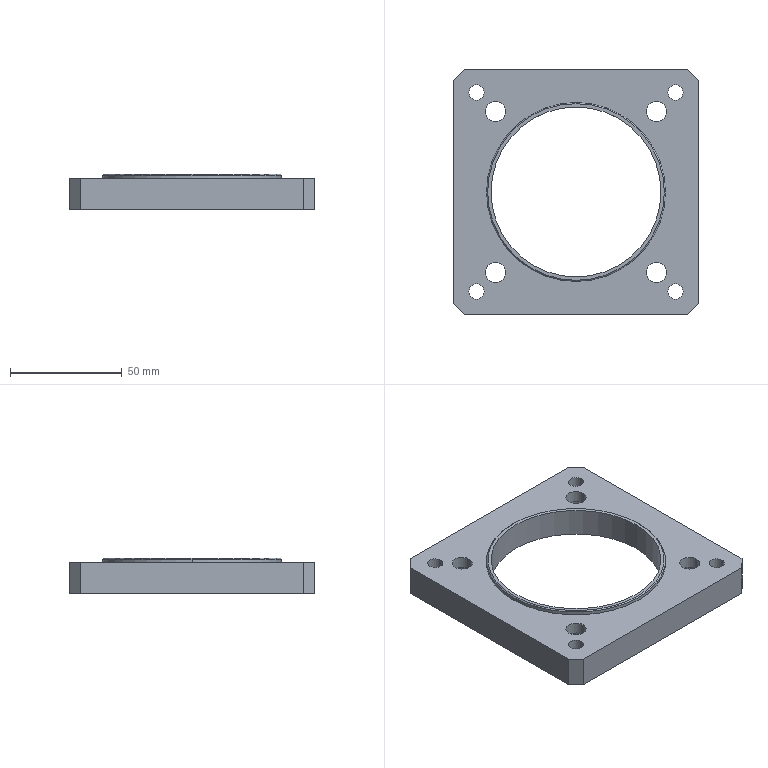Part | SolidWorks | features ICE 3, Chamfer 2, HoleWzd 2, Extrusion 1 | 1 solid | 50 faces | box 110 x 110 x 16 mm | volume 93090 mm3 | cylinder 30 | plane 16 | cone 4 | commonest cylinder face diameters 6.8 x8 9 x8 15 x8 76 x2 80 x2 85 x2
STEP:
#1=CARTESIAN_POINT('',(42.5,0.,0.5));
#2=VERTEX_POINT('',#1);
#3=CARTESIAN_POINT('',(-42.5,0.,0.5));
#4=VERTEX_POINT('',#3);
#5=CARTESIAN_POINT('',(0.,0.,0.5));
#6=DIRECTION('',(0.,0.,-1.));
#7=DIRECTION('',(-1.,0.,0.));
#8=AXIS2_PLACEMENT_3D('',#5,#6,#7);
#9=CIRCLE('',#8,42.5);
#10=EDGE_CURVE('',#2,#4,#9,.T.);
#11=ORIENTED_EDGE('',*,*,#10,.F.);
#12=CARTESIAN_POINT('',(43.,0.,0.));
#13=VERTEX_POINT('',#12);
#14=CARTESIAN_POINT('',(42.5,0.,0.5));
#15=DIRECTION('',(0.7071,0.,-0.7071));
#16=VECTOR('',#15,1000.);
#17=LINE('',#14,#16);
#18=EDGE_CURVE('',#2,#13,#17,.T.);
#19=ORIENTED_EDGE('',*,*,#18,.T.);
#20=CARTESIAN_POINT('',(-43.,0.,0.));
#21=VERTEX_POINT('',#20);
#22=CARTESIAN_POINT('',(0.,0.,0.));
#23=DIRECTION('',(0.,0.,1.));
#24=DIRECTION('',(-1.,0.,0.));
#25=AXIS2_PLACEMENT_3D('',#22,#23,#24);
#26=CIRCLE('',#25,43.);
#27=EDGE_CURVE('',#21,#13,#26,.T.);
#28=ORIENTED_EDGE('',*,*,#27,.F.);
#29=CARTESIAN_POINT('',(-42.5,0.,0.5));
#30=DIRECTION('',(-0.7071,0.,-0.7071));
#31=VECTOR('',#30,1000.);
#32=LINE('',#29,#31);
#33=EDGE_CURVE('',#4,#21,#32,.T.);
#34=ORIENTED_EDGE('',*,*,#33,.F.);
#35=EDGE_LOOP('',(#11,#19,#28,#34));
#36=FACE_OUTER_BOUND('',#35,.T.);
#37=CARTESIAN_POINT('',(0.,0.,0.5));
#38=DIRECTION('',(0.,0.,-1.));
#39=DIRECTION('',(-1.,0.,0.));
#40=AXIS2_PLACEMENT_3D('',#37,#38,#39);
#41=CONICAL_SURFACE('',#40,42.5,0.7854);
#42=ADVANCED_FACE('',(#36),#41,.F.);
#43=CARTESIAN_POINT('',(39.5,0.,16.));
#44=VERTEX_POINT('',#43);
#45=CARTESIAN_POINT('',(-39.5,0.,16.));
#46=VERTEX_POINT('',#45);
#47=CARTESIAN_POINT('',(0.,0.,16.));
#48=DIRECTION('',(0.,0.,1.));
#49=DIRECTION('',(1.,0.,0.));
#50=AXIS2_PLACEMENT_3D('',#47,#48,#49);
#51=CIRCLE('',#50,39.5);
#52=EDGE_CURVE('',#44,#46,#51,.T.);
#53=ORIENTED_EDGE('',*,*,#52,.F.);
#54=CARTESIAN_POINT('',(40.,0.,15.5));
#55=VERTEX_POINT('',#54);
#56=CARTESIAN_POINT('',(39.5,0.,16.));
#57=DIRECTION('',(0.7071,0.,-0.7071));
#58=VECTOR('',#57,1000.);
#59=LINE('',#56,#58);
#60=EDGE_CURVE('',#44,#55,#59,.T.);
#61=ORIENTED_EDGE('',*,*,#60,.T.);
#62=CARTESIAN_POINT('',(-40.,0.,15.5));
#63=VERTEX_POINT('',#62);
#64=CARTESIAN_POINT('',(0.,0.,15.5));
#65=DIRECTION('',(0.,0.,-1.));
#66=DIRECTION('',(1.,0.,0.));
#67=AXIS2_PLACEMENT_3D('',#64,#65,#66);
#68=CIRCLE('',#67,40.);
#69=EDGE_CURVE('',#63,#55,#68,.T.);
#70=ORIENTED_EDGE('',*,*,#69,.F.);
#71=CARTESIAN_POINT('',(-39.5,0.,16.));
#72=DIRECTION('',(-0.7071,0.,-0.7071));
#73=VECTOR('',#72,1000.);
#74=LINE('',#71,#73);
#75=EDGE_CURVE('',#46,#63,#74,.T.);
#76=ORIENTED_EDGE('',*,*,#75,.F.);
#77=EDGE_LOOP('',(#53,#61,#70,#76));
#78=FACE_OUTER_BOUND('',#77,.T.);
#79=CARTESIAN_POINT('',(0.,0.,16.));
#80=DIRECTION('',(0.,0.,-1.));
#81=DIRECTION('',(-1.,0.,0.));
#82=AXIS2_PLACEMENT_3D('',#79,#80,#81);
#83=CONICAL_SURFACE('',#82,39.5,0.7854);
#84=ADVANCED_FACE('',(#78),#83,.T.);
#85=CARTESIAN_POINT('',(-28.5,36.,8.6));
#86=VERTEX_POINT('',#85);
#87=CARTESIAN_POINT('',(-43.5,36.,8.6));
#88=VERTEX_POINT('',#87);
#89=CARTESIAN_POINT('',(-36.,36.,8.6));
#90=DIRECTION('',(0.,0.,-1.));
#91=DIRECTION('',(-1.,0.,0.));
#92=AXIS2_PLACEMENT_3D('',#89,#90,#91);
#93=CIRCLE('',#92,7.5);
#94=EDGE_CURVE('',#86,#88,#93,.T.);
#95=ORIENTED_EDGE('',*,*,#94,.F.);
#96=CARTESIAN_POINT('',(-28.5,36.,0.));
#97=VERTEX_POINT('',#96);
#98=CARTESIAN_POINT('',(-28.5,36.,0.));
#99=DIRECTION('',(0.,0.,-1.));
#100=VECTOR('',#99,1000.);
#101=LINE('',#98,#100);
#102=EDGE_CURVE('',#86,#97,#101,.T.);
#103=ORIENTED_EDGE('',*,*,#102,.T.);
#104=CARTESIAN_POINT('',(-43.5,36.,0.));
#105=VERTEX_POINT('',#104);
#106=CARTESIAN_POINT('',(-36.,36.,0.));
#107=DIRECTION('',(0.,0.,-1.));
#108=DIRECTION('',(-1.,0.,0.));
#109=AXIS2_PLACEMENT_3D('',#106,#107,#108);
#110=CIRCLE('',#109,7.5);
#111=EDGE_CURVE('',#97,#105,#110,.T.);
#112=ORIENTED_EDGE('',*,*,#111,.T.);
#113=CARTESIAN_POINT('',(-43.5,36.,0.));
#114=DIRECTION('',(0.,0.,-1.));
#115=VECTOR('',#114,1000.);
#116=LINE('',#113,#115);
#117=EDGE_CURVE('',#88,#105,#116,.T.);
#118=ORIENTED_EDGE('',*,*,#117,.F.);
#119=EDGE_LOOP('',(#95,#103,#112,#118));
#120=FACE_OUTER_BOUND('',#119,.T.);
#121=CARTESIAN_POINT('',(-36.,36.,0.));
#122=DIRECTION('',(0.,0.,-1.));
#123=DIRECTION('',(-1.,0.,0.));
#124=AXIS2_PLACEMENT_3D('',#121,#122,#123);
#125=CYLINDRICAL_SURFACE('',#124,7.5);
#126=ADVANCED_FACE('',(#120),#125,.F.);
#127=CARTESIAN_POINT('',(-31.5,36.,14.));
#128=VERTEX_POINT('',#127);
#129=CARTESIAN_POINT('',(-40.5,36.,14.));
#130=VERTEX_POINT('',#129);
#131=CARTESIAN_POINT('',(-36.,36.,14.));
#132=DIRECTION('',(0.,0.,-1.));
#133=DIRECTION('',(-1.,0.,0.));
#134=AXIS2_PLACEMENT_3D('',#131,#132,#133);
#135=CIRCLE('',#134,4.5);
#136=EDGE_CURVE('',#128,#130,#135,.T.);
#137=ORIENTED_EDGE('',*,*,#136,.F.);
#138=CARTESIAN_POINT('',(-31.5,36.,8.6));
#139=VERTEX_POINT('',#138);
#140=CARTESIAN_POINT('',(-31.5,36.,0.));
#141=DIRECTION('',(0.,0.,-1.));
#142=VECTOR('',#141,1000.);
#143=LINE('',#140,#142);
#144=EDGE_CURVE('',#128,#139,#143,.T.);
#145=ORIENTED_EDGE('',*,*,#144,.T.);
#146=CARTESIAN_POINT('',(-40.5,36.,8.6));
#147=VERTEX_POINT('',#146);
#148=CARTESIAN_POINT('',(-36.,36.,8.6));
#149=DIRECTION('',(0.,0.,-1.));
#150=DIRECTION('',(-1.,0.,0.));
#151=AXIS2_PLACEMENT_3D('',#148,#149,#150);
#152=CIRCLE('',#151,4.5);
#153=EDGE_CURVE('',#139,#147,#152,.T.);
#154=ORIENTED_EDGE('',*,*,#153,.T.);
#155=CARTESIAN_POINT('',(-40.5,36.,0.));
#156=DIRECTION('',(0.,0.,-1.));
#157=VECTOR('',#156,1000.);
#158=LINE('',#155,#157);
#159=EDGE_CURVE('',#130,#147,#158,.T.);
#160=ORIENTED_EDGE('',*,*,#159,.F.);
#161=EDGE_LOOP('',(#137,#145,#154,#160));
#162=FACE_OUTER_BOUND('',#161,.T.);
#163=CARTESIAN_POINT('',(-36.,36.,0.));
#164=DIRECTION('',(0.,0.,-1.));
#165=DIRECTION('',(-1.,0.,0.));
#166=AXIS2_PLACEMENT_3D('',#163,#164,#165);
#167=CYLINDRICAL_SURFACE('',#166,4.5);
#168=ADVANCED_FACE('',(#162),#167,.F.);
#169=CARTESIAN_POINT('',(43.5,-36.,8.6));
#170=VERTEX_POINT('',#169);
#171=CARTESIAN_POINT('',(28.5,-36.,8.6));
#172=VERTEX_POINT('',#171);
#173=CARTESIAN_POINT('',(36.,-36.,8.6));
#174=DIRECTION('',(0.,0.,-1.));
#175=DIRECTION('',(-1.,0.,0.));
#176=AXIS2_PLACEMENT_3D('',#173,#174,#175);
#177=CIRCLE('',#176,7.5);
#178=EDGE_CURVE('',#170,#172,#177,.T.);
#179=ORIENTED_EDGE('',*,*,#178,.F.);
#180=CARTESIAN_POINT('',(43.5,-36.,0.));
#181=VERTEX_POINT('',#180);
#182=CARTESIAN_POINT('',(43.5,-36.,0.));
#183=DIRECTION('',(0.,0.,-1.));
#184=VECTOR('',#183,1000.);
#185=LINE('',#182,#184);
#186=EDGE_CURVE('',#170,#181,#185,.T.);
#187=ORIENTED_EDGE('',*,*,#186,.T.);
#188=CARTESIAN_POINT('',(28.5,-36.,0.));
#189=VERTEX_POINT('',#188);
#190=CARTESIAN_POINT('',(36.,-36.,0.));
#191=DIRECTION('',(0.,0.,-1.));
#192=DIRECTION('',(-1.,0.,0.));
#193=AXIS2_PLACEMENT_3D('',#190,#191,#192);
#194=CIRCLE('',#193,7.5);
#195=EDGE_CURVE('',#181,#189,#194,.T.);
#196=ORIENTED_EDGE('',*,*,#195,.T.);
#197=CARTESIAN_POINT('',(28.5,-36.,0.));
#198=DIRECTION('',(0.,0.,-1.));
#199=VECTOR('',#198,1000.);
#200=LINE('',#197,#199);
#201=EDGE_CURVE('',#172,#189,#200,.T.);
#202=ORIENTED_EDGE('',*,*,#201,.F.);
#203=EDGE_LOOP('',(#179,#187,#196,#202));
#204=FACE_OUTER_BOUND('',#203,.T.);
#205=CARTESIAN_POINT('',(36.,-36.,0.));
#206=DIRECTION('',(0.,0.,-1.));
#207=DIRECTION('',(-1.,0.,0.));
#208=AXIS2_PLACEMENT_3D('',#205,#206,#207);
#209=CYLINDRICAL_SURFACE('',#208,7.5);
#210=ADVANCED_FACE('',(#204),#209,.F.);
#211=CARTESIAN_POINT('',(40.5,-36.,14.));
#212=VERTEX_POINT('',#211);
#213=CARTESIAN_POINT('',(31.5,-36.,14.));
#214=VERTEX_POINT('',#213);
#215=CARTESIAN_POINT('',(36.,-36.,14.));
#216=DIRECTION('',(0.,0.,-1.));
#217=DIRECTION('',(-1.,0.,0.));
#218=AXIS2_PLACEMENT_3D('',#215,#216,#217);
#219=CIRCLE('',#218,4.5);
#220=EDGE_CURVE('',#212,#214,#219,.T.);
#221=ORIENTED_EDGE('',*,*,#220,.F.);
#222=CARTESIAN_POINT('',(40.5,-36.,8.6));
#223=VERTEX_POINT('',#222);
#224=CARTESIAN_POINT('',(40.5,-36.,0.));
#225=DIRECTION('',(0.,0.,-1.));
#226=VECTOR('',#225,1000.);
#227=LINE('',#224,#226);
#228=EDGE_CURVE('',#212,#223,#227,.T.);
#229=ORIENTED_EDGE('',*,*,#228,.T.);
#230=CARTESIAN_POINT('',(31.5,-36.,8.6));
#231=VERTEX_POINT('',#230);
#232=CARTESIAN_POINT('',(36.,-36.,8.6));
#233=DIRECTION('',(0.,0.,-1.));
#234=DIRECTION('',(-1.,0.,0.));
#235=AXIS2_PLACEMENT_3D('',#232,#233,#234);
#236=CIRCLE('',#235,4.5);
#237=EDGE_CURVE('',#223,#231,#236,.T.);
#238=ORIENTED_EDGE('',*,*,#237,.T.);
#239=CARTESIAN_POINT('',(31.5,-36.,0.));
#240=DIRECTION('',(0.,0.,-1.));
#241=VECTOR('',#240,1000.);
#242=LINE('',#239,#241);
#243=EDGE_CURVE('',#214,#231,#242,.T.);
#244=ORIENTED_EDGE('',*,*,#243,.F.);
#245=EDGE_LOOP('',(#221,#229,#238,#244));
#246=FACE_OUTER_BOUND('',#245,.T.);
#247=CARTESIAN_POINT('',(36.,-36.,0.));
#248=DIRECTION('',(0.,0.,-1.));
#249=DIRECTION('',(-1.,0.,0.));
#250=AXIS2_PLACEMENT_3D('',#247,#248,#249);
#251=CYLINDRICAL_SURFACE('',#250,4.5);
#252=ADVANCED_FACE('',(#246),#251,.F.);
#253=CARTESIAN_POINT('',(43.5,36.,8.6));
#254=VERTEX_POINT('',#253);
#255=CARTESIAN_POINT('',(28.5,36.,8.6));
#256=VERTEX_POINT('',#255);
#257=CARTESIAN_POINT('',(36.,36.,8.6));
#258=DIRECTION('',(0.,0.,-1.));
#259=DIRECTION('',(-1.,0.,0.));
#260=AXIS2_PLACEMENT_3D('',#257,#258,#259);
#261=CIRCLE('',#260,7.5);
#262=EDGE_CURVE('',#254,#256,#261,.T.);
#263=ORIENTED_EDGE('',*,*,#262,.F.);
#264=CARTESIAN_POINT('',(43.5,36.,0.));
#265=VERTEX_POINT('',#264);
#266=CARTESIAN_POINT('',(43.5,36.,0.));
#267=DIRECTION('',(0.,0.,-1.));
#268=VECTOR('',#267,1000.);
#269=LINE('',#266,#268);
#270=EDGE_CURVE('',#254,#265,#269,.T.);
#271=ORIENTED_EDGE('',*,*,#270,.T.);
#272=CARTESIAN_POINT('',(28.5,36.,0.));
#273=VERTEX_POINT('',#272);
#274=CARTESIAN_POINT('',(36.,36.,0.));
#275=DIRECTION('',(0.,0.,-1.));
#276=DIRECTION('',(-1.,0.,0.));
#277=AXIS2_PLACEMENT_3D('',#274,#275,#276);
#278=CIRCLE('',#277,7.5);
#279=EDGE_CURVE('',#265,#273,#278,.T.);
#280=ORIENTED_EDGE('',*,*,#279,.T.);
#281=CARTESIAN_POINT('',(28.5,36.,0.));
#282=DIRECTION('',(0.,0.,-1.));
#283=VECTOR('',#282,1000.);
#284=LINE('',#281,#283);
#285=EDGE_CURVE('',#256,#273,#284,.T.);
#286=ORIENTED_EDGE('',*,*,#285,.F.);
#287=EDGE_LOOP('',(#263,#271,#280,#286));
#288=FACE_OUTER_BOUND('',#287,.T.);
#289=CARTESIAN_POINT('',(36.,36.,0.));
#290=DIRECTION('',(0.,0.,-1.));
#291=DIRECTION('',(-1.,0.,0.));
#292=AXIS2_PLACEMENT_3D('',#289,#290,#291);
#293=CYLINDRICAL_SURFACE('',#292,7.5);
#294=ADVANCED_FACE('',(#288),#293,.F.);
#295=CARTESIAN_POINT('',(40.5,36.,14.));
#296=VERTEX_POINT('',#295);
#297=CARTESIAN_POINT('',(31.5,36.,14.));
#298=VERTEX_POINT('',#297);
#299=CARTESIAN_POINT('',(36.,36.,14.));
#300=DIRECTION('',(0.,0.,-1.));
#301=DIRECTION('',(-1.,0.,0.));
#302=AXIS2_PLACEMENT_3D('',#299,#300,#301);
#303=CIRCLE('',#302,4.5);
#304=EDGE_CURVE('',#296,#298,#303,.T.);
#305=ORIENTED_EDGE('',*,*,#304,.F.);
#306=CARTESIAN_POINT('',(40.5,36.,8.6));
#307=VERTEX_POINT('',#306);
#308=CARTESIAN_POINT('',(40.5,36.,0.));
#309=DIRECTION('',(0.,0.,-1.));
#310=VECTOR('',#309,1000.);
#311=LINE('',#308,#310);
#312=EDGE_CURVE('',#296,#307,#311,.T.);
#313=ORIENTED_EDGE('',*,*,#312,.T.);
#314=CARTESIAN_POINT('',(31.5,36.,8.6));
#315=VERTEX_POINT('',#314);
#316=CARTESIAN_POINT('',(36.,36.,8.6));
#317=DIRECTION('',(0.,0.,-1.));
#318=DIRECTION('',(-1.,0.,0.));
#319=AXIS2_PLACEMENT_3D('',#316,#317,#318);
#320=CIRCLE('',#319,4.5);
#321=EDGE_CURVE('',#307,#315,#320,.T.);
#322=ORIENTED_EDGE('',*,*,#321,.T.);
#323=CARTESIAN_POINT('',(31.5,36.,0.));
#324=DIRECTION('',(0.,0.,-1.));
#325=VECTOR('',#324,1000.);
#326=LINE('',#323,#325);
#327=EDGE_CURVE('',#298,#315,#326,.T.);
#328=ORIENTED_EDGE('',*,*,#327,.F.);
#329=EDGE_LOOP('',(#305,#313,#322,#328));
#330=FACE_OUTER_BOUND('',#329,.T.);
#331=CARTESIAN_POINT('',(36.,36.,0.));
#332=DIRECTION('',(0.,0.,-1.));
#333=DIRECTION('',(-1.,0.,0.));
#334=AXIS2_PLACEMENT_3D('',#331,#332,#333);
#335=CYLINDRICAL_SURFACE('',#334,4.5);
#336=ADVANCED_FACE('',(#330),#335,.F.);
#337=CARTESIAN_POINT('',(-28.5,-36.,8.6));
#338=VERTEX_POINT('',#337);
#339=CARTESIAN_POINT('',(-43.5,-36.,8.6));
#340=VERTEX_POINT('',#339);
#341=CARTESIAN_POINT('',(-36.,-36.,8.6));
#342=DIRECTION('',(0.,0.,-1.));
#343=DIRECTION('',(-1.,0.,0.));
#344=AXIS2_PLACEMENT_3D('',#341,#342,#343);
#345=CIRCLE('',#344,7.5);
#346=EDGE_CURVE('',#338,#340,#345,.T.);
#347=ORIENTED_EDGE('',*,*,#346,.F.);
#348=CARTESIAN_POINT('',(-28.5,-36.,0.));
#349=VERTEX_POINT('',#348);
#350=CARTESIAN_POINT('',(-28.5,-36.,0.));
#351=DIRECTION('',(0.,0.,-1.));
#352=VECTOR('',#351,1000.);
#353=LINE('',#350,#352);
#354=EDGE_CURVE('',#338,#349,#353,.T.);
#355=ORIENTED_EDGE('',*,*,#354,.T.);
#356=CARTESIAN_POINT('',(-43.5,-36.,0.));
#357=VERTEX_POINT('',#356);
#358=CARTESIAN_POINT('',(-36.,-36.,0.));
#359=DIRECTION('',(0.,0.,-1.));
#360=DIRECTION('',(-1.,0.,0.));
#361=AXIS2_PLACEMENT_3D('',#358,#359,#360);
#362=CIRCLE('',#361,7.5);
#363=EDGE_CURVE('',#349,#357,#362,.T.);
#364=ORIENTED_EDGE('',*,*,#363,.T.);
#365=CARTESIAN_POINT('',(-43.5,-36.,0.));
#366=DIRECTION('',(0.,0.,-1.));
#367=VECTOR('',#366,1000.);
#368=LINE('',#365,#367);
#369=EDGE_CURVE('',#340,#357,#368,.T.);
#370=ORIENTED_EDGE('',*,*,#369,.F.);
#371=EDGE_LOOP('',(#347,#355,#364,#370));
#372=FACE_OUTER_BOUND('',#371,.T.);
#373=CARTESIAN_POINT('',(-36.,-36.,0.));
#374=DIRECTION('',(0.,0.,-1.));
#375=DIRECTION('',(-1.,0.,0.));
#376=AXIS2_PLACEMENT_3D('',#373,#374,#375);
#377=CYLINDRICAL_SURFACE('',#376,7.5);
#378=ADVANCED_FACE('',(#372),#377,.F.);
#379=CARTESIAN_POINT('',(-31.5,-36.,14.));
#380=VERTEX_POINT('',#379);
#381=CARTESIAN_POINT('',(-40.5,-36.,14.));
#382=VERTEX_POINT('',#381);
#383=CARTESIAN_POINT('',(-36.,-36.,14.));
#384=DIRECTION('',(0.,0.,-1.));
#385=DIRECTION('',(-1.,0.,0.));
#386=AXIS2_PLACEMENT_3D('',#383,#384,#385);
#387=CIRCLE('',#386,4.5);
#388=EDGE_CURVE('',#380,#382,#387,.T.);
#389=ORIENTED_EDGE('',*,*,#388,.F.);
#390=CARTESIAN_POINT('',(-31.5,-36.,8.6));
#391=VERTEX_POINT('',#390);
#392=CARTESIAN_POINT('',(-31.5,-36.,0.));
#393=DIRECTION('',(0.,0.,-1.));
#394=VECTOR('',#393,1000.);
#395=LINE('',#392,#394);
#396=EDGE_CURVE('',#380,#391,#395,.T.);
#397=ORIENTED_EDGE('',*,*,#396,.T.);
#398=CARTESIAN_POINT('',(-40.5,-36.,8.6));
#399=VERTEX_POINT('',#398);
#400=CARTESIAN_POINT('',(-36.,-36.,8.6));
#401=DIRECTION('',(0.,0.,-1.));
#402=DIRECTION('',(-1.,0.,0.));
#403=AXIS2_PLACEMENT_3D('',#400,#401,#402);
#404=CIRCLE('',#403,4.5);
#405=EDGE_CURVE('',#391,#399,#404,.T.);
#406=ORIENTED_EDGE('',*,*,#405,.T.);
#407=CARTESIAN_POINT('',(-40.5,-36.,0.));
#408=DIRECTION('',(0.,0.,-1.));
#409=VECTOR('',#408,1000.);
#410=LINE('',#407,#409);
#411=EDGE_CURVE('',#382,#399,#410,.T.);
#412=ORIENTED_EDGE('',*,*,#411,.F.);
#413=EDGE_LOOP('',(#389,#397,#406,#412));
#414=FACE_OUTER_BOUND('',#413,.T.);
#415=CARTESIAN_POINT('',(-36.,-36.,0.));
#416=DIRECTION('',(0.,0.,-1.));
#417=DIRECTION('',(-1.,0.,0.));
#418=AXIS2_PLACEMENT_3D('',#415,#416,#417);
#419=CYLINDRICAL_SURFACE('',#418,4.5);
#420=ADVANCED_FACE('',(#414),#419,.F.);
#421=CARTESIAN_POINT('',(47.9,44.5,14.));
#422=VERTEX_POINT('',#421);
#423=CARTESIAN_POINT('',(41.1,44.5,14.));
#424=VERTEX_POINT('',#423);
#425=CARTESIAN_POINT('',(44.5,44.5,14.));
#426=DIRECTION('',(0.,0.,-1.));
#427=DIRECTION('',(-1.,0.,0.));
#428=AXIS2_PLACEMENT_3D('',#425,#426,#427);
#429=CIRCLE('',#428,3.4);
#430=EDGE_CURVE('',#422,#424,#429,.T.);
#431=ORIENTED_EDGE('',*,*,#430,.F.);
#432=CARTESIAN_POINT('',(47.9,44.5,0.));
#433=VERTEX_POINT('',#432);
#434=CARTESIAN_POINT('',(47.9,44.5,0.));
#435=DIRECTION('',(0.,0.,-1.));
#436=VECTOR('',#435,1000.);
#437=LINE('',#434,#436);
#438=EDGE_CURVE('',#422,#433,#437,.T.);
#439=ORIENTED_EDGE('',*,*,#438,.T.);
#440=CARTESIAN_POINT('',(41.1,44.5,0.));
#441=VERTEX_POINT('',#440);
#442=CARTESIAN_POINT('',(44.5,44.5,0.));
#443=DIRECTION('',(0.,0.,-1.));
#444=DIRECTION('',(-1.,0.,0.));
#445=AXIS2_PLACEMENT_3D('',#442,#443,#444);
#446=CIRCLE('',#445,3.4);
#447=EDGE_CURVE('',#433,#441,#446,.T.);
#448=ORIENTED_EDGE('',*,*,#447,.T.);
#449=CARTESIAN_POINT('',(41.1,44.5,0.));
#450=DIRECTION('',(0.,0.,-1.));
#451=VECTOR('',#450,1000.);
#452=LINE('',#449,#451);
#453=EDGE_CURVE('',#424,#441,#452,.T.);
#454=ORIENTED_EDGE('',*,*,#453,.F.);
#455=EDGE_LOOP('',(#431,#439,#448,#454));
#456=FACE_OUTER_BOUND('',#455,.T.);
#457=CARTESIAN_POINT('',(44.5,44.5,0.));
#458=DIRECTION('',(0.,0.,-1.));
#459=DIRECTION('',(-1.,0.,0.));
#460=AXIS2_PLACEMENT_3D('',#457,#458,#459);
#461=CYLINDRICAL_SURFACE('',#460,3.4);
#462=ADVANCED_FACE('',(#456),#461,.F.);
#463=CARTESIAN_POINT('',(-41.1,44.5,14.));
#464=VERTEX_POINT('',#463);
#465=CARTESIAN_POINT('',(-47.9,44.5,14.));
#466=VERTEX_POINT('',#465);
#467=CARTESIAN_POINT('',(-44.5,44.5,14.));
#468=DIRECTION('',(0.,0.,-1.));
#469=DIRECTION('',(-1.,0.,0.));
#470=AXIS2_PLACEMENT_3D('',#467,#468,#469);
#471=CIRCLE('',#470,3.4);
#472=EDGE_CURVE('',#464,#466,#471,.T.);
#473=ORIENTED_EDGE('',*,*,#472,.F.);
#474=CARTESIAN_POINT('',(-41.1,44.5,0.));
#475=VERTEX_POINT('',#474);
#476=CARTESIAN_POINT('',(-41.1,44.5,0.));
#477=DIRECTION('',(0.,0.,-1.));
#478=VECTOR('',#477,1000.);
#479=LINE('',#476,#478);
#480=EDGE_CURVE('',#464,#475,#479,.T.);
#481=ORIENTED_EDGE('',*,*,#480,.T.);
#482=CARTESIAN_POINT('',(-47.9,44.5,0.));
#483=VERTEX_POINT('',#482);
#484=CARTESIAN_POINT('',(-44.5,44.5,0.));
#485=DIRECTION('',(0.,0.,-1.));
#486=DIRECTION('',(-1.,0.,0.));
#487=AXIS2_PLACEMENT_3D('',#484,#485,#486);
#488=CIRCLE('',#487,3.4);
#489=EDGE_CURVE('',#475,#483,#488,.T.);
#490=ORIENTED_EDGE('',*,*,#489,.T.);
#491=CARTESIAN_POINT('',(-47.9,44.5,0.));
#492=DIRECTION('',(0.,0.,-1.));
#493=VECTOR('',#492,1000.);
#494=LINE('',#491,#493);
#495=EDGE_CURVE('',#466,#483,#494,.T.);
#496=ORIENTED_EDGE('',*,*,#495,.F.);
#497=EDGE_LOOP('',(#473,#481,#490,#496));
#498=FACE_OUTER_BOUND('',#497,.T.);
#499=CARTESIAN_POINT('',(-44.5,44.5,0.));
#500=DIRECTION('',(0.,0.,-1.));
#501=DIRECTION('',(-1.,0.,0.));
#502=AXIS2_PLACEMENT_3D('',#499,#500,#501);
#503=CYLINDRICAL_SURFACE('',#502,3.4);
#504=ADVANCED_FACE('',(#498),#503,.F.);
#505=CARTESIAN_POINT('',(47.9,-44.5,14.));
#506=VERTEX_POINT('',#505);
#507=CARTESIAN_POINT('',(41.1,-44.5,14.));
#508=VERTEX_POINT('',#507);
#509=CARTESIAN_POINT('',(44.5,-44.5,14.));
#510=DIRECTION('',(0.,0.,-1.));
#511=DIRECTION('',(-1.,0.,0.));
#512=AXIS2_PLACEMENT_3D('',#509,#510,#511);
#513=CIRCLE('',#512,3.4);
#514=EDGE_CURVE('',#506,#508,#513,.T.);
#515=ORIENTED_EDGE('',*,*,#514,.F.);
#516=CARTESIAN_POINT('',(47.9,-44.5,0.));
#517=VERTEX_POINT('',#516);
#518=CARTESIAN_POINT('',(47.9,-44.5,0.));
#519=DIRECTION('',(0.,0.,-1.));
#520=VECTOR('',#519,1000.);
#521=LINE('',#518,#520);
#522=EDGE_CURVE('',#506,#517,#521,.T.);
#523=ORIENTED_EDGE('',*,*,#522,.T.);
#524=CARTESIAN_POINT('',(41.1,-44.5,0.));
#525=VERTEX_POINT('',#524);
#526=CARTESIAN_POINT('',(44.5,-44.5,0.));
#527=DIRECTION('',(0.,0.,-1.));
#528=DIRECTION('',(-1.,0.,0.));
#529=AXIS2_PLACEMENT_3D('',#526,#527,#528);
#530=CIRCLE('',#529,3.4);
#531=EDGE_CURVE('',#517,#525,#530,.T.);
#532=ORIENTED_EDGE('',*,*,#531,.T.);
#533=CARTESIAN_POINT('',(41.1,-44.5,0.));
#534=DIRECTION('',(0.,0.,-1.));
#535=VECTOR('',#534,1000.);
#536=LINE('',#533,#535);
#537=EDGE_CURVE('',#508,#525,#536,.T.);
#538=ORIENTED_EDGE('',*,*,#537,.F.);
#539=EDGE_LOOP('',(#515,#523,#532,#538));
#540=FACE_OUTER_BOUND('',#539,.T.);
#541=CARTESIAN_POINT('',(44.5,-44.5,0.));
#542=DIRECTION('',(0.,0.,-1.));
#543=DIRECTION('',(-1.,0.,0.));
#544=AXIS2_PLACEMENT_3D('',#541,#542,#543);
#545=CYLINDRICAL_SURFACE('',#544,3.4);
#546=ADVANCED_FACE('',(#540),#545,.F.);
#547=CARTESIAN_POINT('',(-41.1,-44.5,14.));
#548=VERTEX_POINT('',#547);
#549=CARTESIAN_POINT('',(-47.9,-44.5,14.));
#550=VERTEX_POINT('',#549);
#551=CARTESIAN_POINT('',(-44.5,-44.5,14.));
#552=DIRECTION('',(0.,0.,-1.));
#553=DIRECTION('',(-1.,0.,0.));
#554=AXIS2_PLACEMENT_3D('',#551,#552,#553);
#555=CIRCLE('',#554,3.4);
#556=EDGE_CURVE('',#548,#550,#555,.T.);
#557=ORIENTED_EDGE('',*,*,#556,.F.);
#558=CARTESIAN_POINT('',(-41.1,-44.5,0.));
#559=VERTEX_POINT('',#558);
#560=CARTESIAN_POINT('',(-41.1,-44.5,0.));
#561=DIRECTION('',(0.,0.,-1.));
#562=VECTOR('',#561,1000.);
#563=LINE('',#560,#562);
#564=EDGE_CURVE('',#548,#559,#563,.T.);
#565=ORIENTED_EDGE('',*,*,#564,.T.);
#566=CARTESIAN_POINT('',(-47.9,-44.5,0.));
#567=VERTEX_POINT('',#566);
#568=CARTESIAN_POINT('',(-44.5,-44.5,0.));
#569=DIRECTION('',(0.,0.,-1.));
#570=DIRECTION('',(-1.,0.,0.));
#571=AXIS2_PLACEMENT_3D('',#568,#569,#570);
#572=CIRCLE('',#571,3.4);
#573=EDGE_CURVE('',#559,#567,#572,.T.);
#574=ORIENTED_EDGE('',*,*,#573,.T.);
#575=CARTESIAN_POINT('',(-47.9,-44.5,0.));
#576=DIRECTION('',(0.,0.,-1.));
#577=VECTOR('',#576,1000.);
#578=LINE('',#575,#577);
#579=EDGE_CURVE('',#550,#567,#578,.T.);
#580=ORIENTED_EDGE('',*,*,#579,.F.);
#581=EDGE_LOOP('',(#557,#565,#574,#580));
#582=FACE_OUTER_BOUND('',#581,.T.);
#583=CARTESIAN_POINT('',(-44.5,-44.5,0.));
#584=DIRECTION('',(0.,0.,-1.));
#585=DIRECTION('',(-1.,0.,0.));
#586=AXIS2_PLACEMENT_3D('',#583,#584,#585);
#587=CYLINDRICAL_SURFACE('',#586,3.4);
#588=ADVANCED_FACE('',(#582),#587,.F.);
#589=CARTESIAN_POINT('',(42.5,0.,3.1));
#590=VERTEX_POINT('',#589);
#591=CARTESIAN_POINT('',(-42.5,0.,3.1));
#592=VERTEX_POINT('',#591);
#593=CARTESIAN_POINT('',(0.,0.,3.1));
#594=DIRECTION('',(0.,0.,-1.));
#595=DIRECTION('',(-1.,0.,0.));
#596=AXIS2_PLACEMENT_3D('',#593,#594,#595);
#597=CIRCLE('',#596,42.5);
#598=EDGE_CURVE('',#590,#592,#597,.T.);
#599=ORIENTED_EDGE('',*,*,#598,.F.);
#600=CARTESIAN_POINT('',(42.5,0.,3.1));
#601=DIRECTION('',(0.,0.,-1.));
#602=VECTOR('',#601,1000.);
#603=LINE('',#600,#602);
#604=EDGE_CURVE('',#590,#2,#603,.T.);
#605=ORIENTED_EDGE('',*,*,#604,.T.);
#606=ORIENTED_EDGE('',*,*,#10,.T.);
#607=CARTESIAN_POINT('',(-42.5,0.,3.1));
#608=DIRECTION('',(0.,0.,-1.));
#609=VECTOR('',#608,1000.);
#610=LINE('',#607,#609);
#611=EDGE_CURVE('',#592,#4,#610,.T.);
#612=ORIENTED_EDGE('',*,*,#611,.F.);
#613=EDGE_LOOP('',(#599,#605,#606,#612));
#614=FACE_OUTER_BOUND('',#613,.T.);
#615=CARTESIAN_POINT('',(0.,0.,3.1));
#616=DIRECTION('',(0.,0.,-1.));
#617=DIRECTION('',(-1.,0.,0.));
#618=AXIS2_PLACEMENT_3D('',#615,#616,#617);
#619=CYLINDRICAL_SURFACE('',#618,42.5);
#620=ADVANCED_FACE('',(#614),#619,.F.);
#621=ORIENTED_EDGE('',*,*,#69,.T.);
#622=CARTESIAN_POINT('',(40.,0.,14.));
#623=VERTEX_POINT('',#622);
#624=CARTESIAN_POINT('',(40.,0.,16.));
#625=DIRECTION('',(0.,0.,-1.));
#626=VECTOR('',#625,1000.);
#627=LINE('',#624,#626);
#628=EDGE_CURVE('',#55,#623,#627,.T.);
#629=ORIENTED_EDGE('',*,*,#628,.T.);
#630=CARTESIAN_POINT('',(-40.,0.,14.));
#631=VERTEX_POINT('',#630);
#632=CARTESIAN_POINT('',(0.,0.,14.));
#633=DIRECTION('',(0.,0.,1.));
#634=DIRECTION('',(-1.,0.,0.));
#635=AXIS2_PLACEMENT_3D('',#632,#633,#634);
#636=CIRCLE('',#635,40.);
#637=EDGE_CURVE('',#623,#631,#636,.T.);
#638=ORIENTED_EDGE('',*,*,#637,.T.);
#639=CARTESIAN_POINT('',(-40.,0.,16.));
#640=DIRECTION('',(0.,0.,-1.));
#641=VECTOR('',#640,1000.);
#642=LINE('',#639,#641);
#643=EDGE_CURVE('',#63,#631,#642,.T.);
#644=ORIENTED_EDGE('',*,*,#643,.F.);
#645=EDGE_LOOP('',(#621,#629,#638,#644));
#646=FACE_OUTER_BOUND('',#645,.T.);
#647=CARTESIAN_POINT('',(0.,0.,16.));
#648=DIRECTION('',(0.,0.,-1.));
#649=DIRECTION('',(-1.,0.,0.));
#650=AXIS2_PLACEMENT_3D('',#647,#648,#649);
#651=CYLINDRICAL_SURFACE('',#650,40.);
#652=ADVANCED_FACE('',(#646),#651,.T.);
#653=CARTESIAN_POINT('',(-38.,0.,16.));
#654=VERTEX_POINT('',#653);
#655=CARTESIAN_POINT('',(38.,0.,16.));
#656=VERTEX_POINT('',#655);
#657=CARTESIAN_POINT('',(0.,0.,16.));
#658=DIRECTION('',(0.,0.,1.));
#659=DIRECTION('',(1.,0.,0.));
#660=AXIS2_PLACEMENT_3D('',#657,#658,#659);
#661=CIRCLE('',#660,38.);
#662=EDGE_CURVE('',#654,#656,#661,.T.);
#663=ORIENTED_EDGE('',*,*,#662,.T.);
#664=CARTESIAN_POINT('',(38.,0.,3.1));
#665=VERTEX_POINT('',#664);
#666=CARTESIAN_POINT('',(38.,0.,16.));
#667=DIRECTION('',(0.,0.,-1.));
#668=VECTOR('',#667,1000.);
#669=LINE('',#666,#668);
#670=EDGE_CURVE('',#656,#665,#669,.T.);
#671=ORIENTED_EDGE('',*,*,#670,.T.);
#672=CARTESIAN_POINT('',(-38.,0.,3.1));
#673=VERTEX_POINT('',#672);
#674=CARTESIAN_POINT('',(0.,0.,3.1));
#675=DIRECTION('',(0.,0.,-1.));
#676=DIRECTION('',(-1.,0.,0.));
#677=AXIS2_PLACEMENT_3D('',#674,#675,#676);
#678=CIRCLE('',#677,38.);
#679=EDGE_CURVE('',#665,#673,#678,.T.);
#680=ORIENTED_EDGE('',*,*,#679,.T.);
#681=CARTESIAN_POINT('',(-38.,0.,16.));
#682=DIRECTION('',(0.,0.,-1.));
#683=VECTOR('',#682,1000.);
#684=LINE('',#681,#683);
#685=EDGE_CURVE('',#654,#673,#684,.T.);
#686=ORIENTED_EDGE('',*,*,#685,.F.);
#687=EDGE_LOOP('',(#663,#671,#680,#686));
#688=FACE_OUTER_BOUND('',#687,.T.);
#689=CARTESIAN_POINT('',(0.,0.,16.));
#690=DIRECTION('',(0.,0.,-1.));
#691=DIRECTION('',(-1.,0.,0.));
#692=AXIS2_PLACEMENT_3D('',#689,#690,#691);
#693=CYLINDRICAL_SURFACE('',#692,38.);
#694=ADVANCED_FACE('',(#688),#693,.F.);
#695=ORIENTED_EDGE('',*,*,#670,.F.);
#696=CARTESIAN_POINT('',(0.,0.,16.));
#697=DIRECTION('',(0.,0.,1.));
#698=DIRECTION('',(1.,0.,0.));
#699=AXIS2_PLACEMENT_3D('',#696,#697,#698);
#700=CIRCLE('',#699,38.);
#701=EDGE_CURVE('',#656,#654,#700,.T.);
#702=ORIENTED_EDGE('',*,*,#701,.T.);
#703=ORIENTED_EDGE('',*,*,#685,.T.);
#704=CARTESIAN_POINT('',(0.,0.,3.1));
#705=DIRECTION('',(0.,0.,-1.));
#706=DIRECTION('',(-1.,0.,0.));
#707=AXIS2_PLACEMENT_3D('',#704,#705,#706);
#708=CIRCLE('',#707,38.);
#709=EDGE_CURVE('',#673,#665,#708,.T.);
#710=ORIENTED_EDGE('',*,*,#709,.T.);
#711=EDGE_LOOP('',(#695,#702,#703,#710));
#712=FACE_OUTER_BOUND('',#711,.T.);
#713=CARTESIAN_POINT('',(0.,0.,16.));
#714=DIRECTION('',(0.,0.,-1.));
#715=DIRECTION('',(-1.,0.,0.));
#716=AXIS2_PLACEMENT_3D('',#713,#714,#715);
#717=CYLINDRICAL_SURFACE('',#716,38.);
#718=ADVANCED_FACE('',(#712),#717,.F.);
#719=CARTESIAN_POINT('',(55.,-50.,14.));
#720=VERTEX_POINT('',#719);
#721=CARTESIAN_POINT('',(55.,50.,14.));
#722=VERTEX_POINT('',#721);
#723=CARTESIAN_POINT('',(55.,-55.,14.));
#724=DIRECTION('',(0.,1.,0.));
#725=VECTOR('',#724,1000.);
#726=LINE('',#723,#725);
#727=EDGE_CURVE('',#720,#722,#726,.T.);
#728=ORIENTED_EDGE('',*,*,#727,.F.);
#729=CARTESIAN_POINT('',(55.,-50.,0.));
#730=VERTEX_POINT('',#729);
#731=CARTESIAN_POINT('',(55.,-50.,14.));
#732=DIRECTION('',(0.,0.,-1.));
#733=VECTOR('',#732,1000.);
#734=LINE('',#731,#733);
#735=EDGE_CURVE('',#720,#730,#734,.T.);
#736=ORIENTED_EDGE('',*,*,#735,.T.);
#737=CARTESIAN_POINT('',(55.,50.,0.));
#738=VERTEX_POINT('',#737);
#739=CARTESIAN_POINT('',(55.,-55.,0.));
#740=DIRECTION('',(0.,1.,0.));
#741=VECTOR('',#740,1000.);
#742=LINE('',#739,#741);
#743=EDGE_CURVE('',#730,#738,#742,.T.);
#744=ORIENTED_EDGE('',*,*,#743,.T.);
#745=CARTESIAN_POINT('',(55.,50.,14.));
#746=DIRECTION('',(0.,0.,1.));
#747=VECTOR('',#746,1000.);
#748=LINE('',#745,#747);
#749=EDGE_CURVE('',#738,#722,#748,.T.);
#750=ORIENTED_EDGE('',*,*,#749,.T.);
#751=EDGE_LOOP('',(#728,#736,#744,#750));
#752=FACE_OUTER_BOUND('',#751,.T.);
#753=CARTESIAN_POINT('',(55.,-55.,14.));
#754=DIRECTION('',(-1.,0.,0.));
#755=DIRECTION('',(0.,0.,1.));
#756=AXIS2_PLACEMENT_3D('',#753,#754,#755);
#757=PLANE('',#756);
#758=ADVANCED_FACE('',(#752),#757,.F.);
#759=CARTESIAN_POINT('',(50.,55.,0.));
#760=VERTEX_POINT('',#759);
#761=CARTESIAN_POINT('',(-50.,55.,0.));
#762=VERTEX_POINT('',#761);
#763=CARTESIAN_POINT('',(-55.,55.,0.));
#764=DIRECTION('',(-1.,0.,0.));
#765=VECTOR('',#764,1000.);
#766=LINE('',#763,#765);
#767=EDGE_CURVE('',#760,#762,#766,.T.);
#768=ORIENTED_EDGE('',*,*,#767,.T.);
#769=CARTESIAN_POINT('',(-50.,55.,14.));
#770=VERTEX_POINT('',#769);
#771=CARTESIAN_POINT('',(-50.,55.,14.));
#772=DIRECTION('',(0.,0.,1.));
#773=VECTOR('',#772,1000.);
#774=LINE('',#771,#773);
#775=EDGE_CURVE('',#762,#770,#774,.T.);
#776=ORIENTED_EDGE('',*,*,#775,.T.);
#777=CARTESIAN_POINT('',(50.,55.,14.));
#778=VERTEX_POINT('',#777);
#779=CARTESIAN_POINT('',(-55.,55.,14.));
#780=DIRECTION('',(-1.,0.,0.));
#781=VECTOR('',#780,1000.);
#782=LINE('',#779,#781);
#783=EDGE_CURVE('',#778,#770,#782,.T.);
#784=ORIENTED_EDGE('',*,*,#783,.F.);
#785=CARTESIAN_POINT('',(50.,55.,14.));
#786=DIRECTION('',(0.,0.,-1.));
#787=VECTOR('',#786,1000.);
#788=LINE('',#785,#787);
#789=EDGE_CURVE('',#778,#760,#788,.T.);
#790=ORIENTED_EDGE('',*,*,#789,.T.);
#791=EDGE_LOOP('',(#768,#776,#784,#790));
#792=FACE_OUTER_BOUND('',#791,.T.);
#793=CARTESIAN_POINT('',(-55.,55.,14.));
#794=DIRECTION('',(0.,-1.,0.));
#795=DIRECTION('',(0.,0.,-1.));
#796=AXIS2_PLACEMENT_3D('',#793,#794,#795);
#797=PLANE('',#796);
#798=ADVANCED_FACE('',(#792),#797,.F.);
#799=CARTESIAN_POINT('',(-55.,50.,0.));
#800=VERTEX_POINT('',#799);
#801=CARTESIAN_POINT('',(-55.,-50.,0.));
#802=VERTEX_POINT('',#801);
#803=CARTESIAN_POINT('',(-55.,-55.,0.));
#804=DIRECTION('',(0.,-1.,0.));
#805=VECTOR('',#804,1000.);
#806=LINE('',#803,#805);
#807=EDGE_CURVE('',#800,#802,#806,.T.);
#808=ORIENTED_EDGE('',*,*,#807,.T.);
#809=CARTESIAN_POINT('',(-55.,-50.,14.));
#810=VERTEX_POINT('',#809);
#811=CARTESIAN_POINT('',(-55.,-50.,14.));
#812=DIRECTION('',(0.,0.,1.));
#813=VECTOR('',#812,1000.);
#814=LINE('',#811,#813);
#815=EDGE_CURVE('',#802,#810,#814,.T.);
#816=ORIENTED_EDGE('',*,*,#815,.T.);
#817=CARTESIAN_POINT('',(-55.,50.,14.));
#818=VERTEX_POINT('',#817);
#819=CARTESIAN_POINT('',(-55.,-55.,14.));
#820=DIRECTION('',(0.,-1.,0.));
#821=VECTOR('',#820,1000.);
#822=LINE('',#819,#821);
#823=EDGE_CURVE('',#818,#810,#822,.T.);
#824=ORIENTED_EDGE('',*,*,#823,.F.);
#825=CARTESIAN_POINT('',(-55.,50.,14.));
#826=DIRECTION('',(0.,0.,-1.));
#827=VECTOR('',#826,1000.);
#828=LINE('',#825,#827);
#829=EDGE_CURVE('',#818,#800,#828,.T.);
#830=ORIENTED_EDGE('',*,*,#829,.T.);
#831=EDGE_LOOP('',(#808,#816,#824,#830));
#832=FACE_OUTER_BOUND('',#831,.T.);
#833=CARTESIAN_POINT('',(-55.,-55.,14.));
#834=DIRECTION('',(1.,0.,0.));
#835=DIRECTION('',(0.,0.,-1.));
#836=AXIS2_PLACEMENT_3D('',#833,#834,#835);
#837=PLANE('',#836);
#838=ADVANCED_FACE('',(#832),#837,.F.);
#839=CARTESIAN_POINT('',(-50.,-55.,0.));
#840=VERTEX_POINT('',#839);
#841=CARTESIAN_POINT('',(50.,-55.,0.));
#842=VERTEX_POINT('',#841);
#843=CARTESIAN_POINT('',(-55.,-55.,0.));
#844=DIRECTION('',(1.,0.,0.));
#845=VECTOR('',#844,1000.);
#846=LINE('',#843,#845);
#847=EDGE_CURVE('',#840,#842,#846,.T.);
#848=ORIENTED_EDGE('',*,*,#847,.T.);
#849=CARTESIAN_POINT('',(50.,-55.,14.));
#850=VERTEX_POINT('',#849);
#851=CARTESIAN_POINT('',(50.,-55.,14.));
#852=DIRECTION('',(0.,0.,1.));
#853=VECTOR('',#852,1000.);
#854=LINE('',#851,#853);
#855=EDGE_CURVE('',#842,#850,#854,.T.);
#856=ORIENTED_EDGE('',*,*,#855,.T.);
#857=CARTESIAN_POINT('',(-50.,-55.,14.));
#858=VERTEX_POINT('',#857);
#859=CARTESIAN_POINT('',(-55.,-55.,14.));
#860=DIRECTION('',(1.,0.,0.));
#861=VECTOR('',#860,1000.);
#862=LINE('',#859,#861);
#863=EDGE_CURVE('',#858,#850,#862,.T.);
#864=ORIENTED_EDGE('',*,*,#863,.F.);
#865=CARTESIAN_POINT('',(-50.,-55.,14.));
#866=DIRECTION('',(0.,0.,-1.));
#867=VECTOR('',#866,1000.);
#868=LINE('',#865,#867);
#869=EDGE_CURVE('',#858,#840,#868,.T.);
#870=ORIENTED_EDGE('',*,*,#869,.T.);
#871=EDGE_LOOP('',(#848,#856,#864,#870));
#872=FACE_OUTER_BOUND('',#871,.T.);
#873=CARTESIAN_POINT('',(-55.,-55.,14.));
#874=DIRECTION('',(0.,1.,0.));
#875=DIRECTION('',(0.,0.,1.));
#876=AXIS2_PLACEMENT_3D('',#873,#874,#875);
#877=PLANE('',#876);
#878=ADVANCED_FACE('',(#872),#877,.F.);
#879=CARTESIAN_POINT('',(-36.,36.,14.));
#880=DIRECTION('',(0.,0.,-1.));
#881=DIRECTION('',(-1.,0.,0.));
#882=AXIS2_PLACEMENT_3D('',#879,#880,#881);
#883=CIRCLE('',#882,4.5);
#884=EDGE_CURVE('',#130,#128,#883,.T.);
#885=ORIENTED_EDGE('',*,*,#884,.T.);
#886=ORIENTED_EDGE('',*,*,#136,.T.);
#887=EDGE_LOOP('',(#885,#886));
#888=FACE_BOUND('',#887,.T.);
#889=CARTESIAN_POINT('',(36.,-36.,14.));
#890=DIRECTION('',(0.,0.,-1.));
#891=DIRECTION('',(-1.,0.,0.));
#892=AXIS2_PLACEMENT_3D('',#889,#890,#891);
#893=CIRCLE('',#892,4.5);
#894=EDGE_CURVE('',#214,#212,#893,.T.);
#895=ORIENTED_EDGE('',*,*,#894,.T.);
#896=ORIENTED_EDGE('',*,*,#220,.T.);
#897=EDGE_LOOP('',(#895,#896));
#898=FACE_BOUND('',#897,.T.);
#899=CARTESIAN_POINT('',(36.,36.,14.));
#900=DIRECTION('',(0.,0.,-1.));
#901=DIRECTION('',(-1.,0.,0.));
#902=AXIS2_PLACEMENT_3D('',#899,#900,#901);
#903=CIRCLE('',#902,4.5);
#904=EDGE_CURVE('',#298,#296,#903,.T.);
#905=ORIENTED_EDGE('',*,*,#904,.T.);
#906=ORIENTED_EDGE('',*,*,#304,.T.);
#907=EDGE_LOOP('',(#905,#906));
#908=FACE_BOUND('',#907,.T.);
#909=CARTESIAN_POINT('',(-36.,-36.,14.));
#910=DIRECTION('',(0.,0.,-1.));
#911=DIRECTION('',(-1.,0.,0.));
#912=AXIS2_PLACEMENT_3D('',#909,#910,#911);
#913=CIRCLE('',#912,4.5);
#914=EDGE_CURVE('',#382,#380,#913,.T.);
#915=ORIENTED_EDGE('',*,*,#914,.T.);
#916=ORIENTED_EDGE('',*,*,#388,.T.);
#917=EDGE_LOOP('',(#915,#916));
#918=FACE_BOUND('',#917,.T.);
#919=CARTESIAN_POINT('',(44.5,44.5,14.));
#920=DIRECTION('',(0.,0.,-1.));
#921=DIRECTION('',(-1.,0.,0.));
#922=AXIS2_PLACEMENT_3D('',#919,#920,#921);
#923=CIRCLE('',#922,3.4);
#924=EDGE_CURVE('',#424,#422,#923,.T.);
#925=ORIENTED_EDGE('',*,*,#924,.T.);
#926=ORIENTED_EDGE('',*,*,#430,.T.);
#927=EDGE_LOOP('',(#925,#926));
#928=FACE_BOUND('',#927,.T.);
#929=CARTESIAN_POINT('',(-44.5,44.5,14.));
#930=DIRECTION('',(0.,0.,-1.));
#931=DIRECTION('',(-1.,0.,0.));
#932=AXIS2_PLACEMENT_3D('',#929,#930,#931);
#933=CIRCLE('',#932,3.4);
#934=EDGE_CURVE('',#466,#464,#933,.T.);
#935=ORIENTED_EDGE('',*,*,#934,.T.);
#936=ORIENTED_EDGE('',*,*,#472,.T.);
#937=EDGE_LOOP('',(#935,#936));
#938=FACE_BOUND('',#937,.T.);
#939=CARTESIAN_POINT('',(44.5,-44.5,14.));
#940=DIRECTION('',(0.,0.,-1.));
#941=DIRECTION('',(-1.,0.,0.));
#942=AXIS2_PLACEMENT_3D('',#939,#940,#941);
#943=CIRCLE('',#942,3.4);
#944=EDGE_CURVE('',#508,#506,#943,.T.);
#945=ORIENTED_EDGE('',*,*,#944,.T.);
#946=ORIENTED_EDGE('',*,*,#514,.T.);
#947=EDGE_LOOP('',(#945,#946));
#948=FACE_BOUND('',#947,.T.);
#949=CARTESIAN_POINT('',(-44.5,-44.5,14.));
#950=DIRECTION('',(0.,0.,-1.));
#951=DIRECTION('',(-1.,0.,0.));
#952=AXIS2_PLACEMENT_3D('',#949,#950,#951);
#953=CIRCLE('',#952,3.4);
#954=EDGE_CURVE('',#550,#548,#953,.T.);
#955=ORIENTED_EDGE('',*,*,#954,.T.);
#956=ORIENTED_EDGE('',*,*,#556,.T.);
#957=EDGE_LOOP('',(#955,#956));
#958=FACE_BOUND('',#957,.T.);
#959=CARTESIAN_POINT('',(0.,0.,14.));
#960=DIRECTION('',(0.,0.,1.));
#961=DIRECTION('',(-1.,0.,0.));
#962=AXIS2_PLACEMENT_3D('',#959,#960,#961);
#963=CIRCLE('',#962,40.);
#964=EDGE_CURVE('',#631,#623,#963,.T.);
#965=ORIENTED_EDGE('',*,*,#964,.F.);
#966=ORIENTED_EDGE('',*,*,#637,.F.);
#967=EDGE_LOOP('',(#965,#966));
#968=FACE_BOUND('',#967,.T.);
#969=ORIENTED_EDGE('',*,*,#863,.T.);
#970=CARTESIAN_POINT('',(55.,-50.,14.));
#971=DIRECTION('',(0.7071,0.7071,0.));
#972=VECTOR('',#971,1000.);
#973=LINE('',#970,#972);
#974=EDGE_CURVE('',#850,#720,#973,.T.);
#975=ORIENTED_EDGE('',*,*,#974,.T.);
#976=ORIENTED_EDGE('',*,*,#727,.T.);
#977=CARTESIAN_POINT('',(50.,55.,14.));
#978=DIRECTION('',(-0.7071,0.7071,0.));
#979=VECTOR('',#978,1000.);
#980=LINE('',#977,#979);
#981=EDGE_CURVE('',#722,#778,#980,.T.);
#982=ORIENTED_EDGE('',*,*,#981,.T.);
#983=ORIENTED_EDGE('',*,*,#783,.T.);
#984=CARTESIAN_POINT('',(-55.,50.,14.));
#985=DIRECTION('',(-0.7071,-0.7071,0.));
#986=VECTOR('',#985,1000.);
#987=LINE('',#984,#986);
#988=EDGE_CURVE('',#770,#818,#987,.T.);
#989=ORIENTED_EDGE('',*,*,#988,.T.);
#990=ORIENTED_EDGE('',*,*,#823,.T.);
#991=CARTESIAN_POINT('',(-50.,-55.,14.));
#992=DIRECTION('',(0.7071,-0.7071,0.));
#993=VECTOR('',#992,1000.);
#994=LINE('',#991,#993);
#995=EDGE_CURVE('',#810,#858,#994,.T.);
#996=ORIENTED_EDGE('',*,*,#995,.T.);
#997=EDGE_LOOP('',(#969,#975,#976,#982,#983,#989,#990,#996));
#998=FACE_OUTER_BOUND('',#997,.T.);
#999=CARTESIAN_POINT('',(0.,0.,14.));
#1000=DIRECTION('',(0.,0.,-1.));
#1001=DIRECTION('',(-1.,0.,0.));
#1002=AXIS2_PLACEMENT_3D('',#999,#1000,#1001);
#1003=PLANE('',#1002);
#1004=ADVANCED_FACE('',(#888,#898,#908,#918,#928,#938,#948,#958,#968,#998),#1003,.F.);
#1005=ORIENTED_EDGE('',*,*,#27,.T.);
#1006=CARTESIAN_POINT('',(0.,0.,0.));
#1007=DIRECTION('',(0.,0.,1.));
#1008=DIRECTION('',(-1.,0.,0.));
#1009=AXIS2_PLACEMENT_3D('',#1006,#1007,#1008);
#1010=CIRCLE('',#1009,43.);
#1011=EDGE_CURVE('',#13,#21,#1010,.T.);
#1012=ORIENTED_EDGE('',*,*,#1011,.T.);
#1013=EDGE_LOOP('',(#1005,#1012));
#1014=FACE_BOUND('',#1013,.T.);
#1015=CARTESIAN_POINT('',(-36.,36.,0.));
#1016=DIRECTION('',(0.,0.,-1.));
#1017=DIRECTION('',(-1.,0.,0.));
#1018=AXIS2_PLACEMENT_3D('',#1015,#1016,#1017);
#1019=CIRCLE('',#1018,7.5);
#1020=EDGE_CURVE('',#105,#97,#1019,.T.);
#1021=ORIENTED_EDGE('',*,*,#1020,.F.);
#1022=ORIENTED_EDGE('',*,*,#111,.F.);
#1023=EDGE_LOOP('',(#1021,#1022));
#1024=FACE_BOUND('',#1023,.T.);
#1025=CARTESIAN_POINT('',(36.,-36.,0.));
#1026=DIRECTION('',(0.,0.,-1.));
#1027=DIRECTION('',(-1.,0.,0.));
#1028=AXIS2_PLACEMENT_3D('',#1025,#1026,#1027);
#1029=CIRCLE('',#1028,7.5);
#1030=EDGE_CURVE('',#189,#181,#1029,.T.);
#1031=ORIENTED_EDGE('',*,*,#1030,.F.);
#1032=ORIENTED_EDGE('',*,*,#195,.F.);
#1033=EDGE_LOOP('',(#1031,#1032));
#1034=FACE_BOUND('',#1033,.T.);
#1035=CARTESIAN_POINT('',(36.,36.,0.));
#1036=DIRECTION('',(0.,0.,-1.));
#1037=DIRECTION('',(-1.,0.,0.));
#1038=AXIS2_PLACEMENT_3D('',#1035,#1036,#1037);
#1039=CIRCLE('',#1038,7.5);
#1040=EDGE_CURVE('',#273,#265,#1039,.T.);
#1041=ORIENTED_EDGE('',*,*,#1040,.F.);
#1042=ORIENTED_EDGE('',*,*,#279,.F.);
#1043=EDGE_LOOP('',(#1041,#1042));
#1044=FACE_BOUND('',#1043,.T.);
#1045=CARTESIAN_POINT('',(-36.,-36.,0.));
#1046=DIRECTION('',(0.,0.,-1.));
#1047=DIRECTION('',(-1.,0.,0.));
#1048=AXIS2_PLACEMENT_3D('',#1045,#1046,#1047);
#1049=CIRCLE('',#1048,7.5);
#1050=EDGE_CURVE('',#357,#349,#1049,.T.);
#1051=ORIENTED_EDGE('',*,*,#1050,.F.);
#1052=ORIENTED_EDGE('',*,*,#363,.F.);
#1053=EDGE_LOOP('',(#1051,#1052));
#1054=FACE_BOUND('',#1053,.T.);
#1055=CARTESIAN_POINT('',(44.5,44.5,0.));
#1056=DIRECTION('',(0.,0.,-1.));
#1057=DIRECTION('',(-1.,0.,0.));
#1058=AXIS2_PLACEMENT_3D('',#1055,#1056,#1057);
#1059=CIRCLE('',#1058,3.4);
#1060=EDGE_CURVE('',#441,#433,#1059,.T.);
#1061=ORIENTED_EDGE('',*,*,#1060,.F.);
#1062=ORIENTED_EDGE('',*,*,#447,.F.);
#1063=EDGE_LOOP('',(#1061,#1062));
#1064=FACE_BOUND('',#1063,.T.);
#1065=CARTESIAN_POINT('',(-44.5,44.5,0.));
#1066=DIRECTION('',(0.,0.,-1.));
#1067=DIRECTION('',(-1.,0.,0.));
#1068=AXIS2_PLACEMENT_3D('',#1065,#1066,#1067);
#1069=CIRCLE('',#1068,3.4);
#1070=EDGE_CURVE('',#483,#475,#1069,.T.);
#1071=ORIENTED_EDGE('',*,*,#1070,.F.);
#1072=ORIENTED_EDGE('',*,*,#489,.F.);
#1073=EDGE_LOOP('',(#1071,#1072));
#1074=FACE_BOUND('',#1073,.T.);
#1075=CARTESIAN_POINT('',(44.5,-44.5,0.));
#1076=DIRECTION('',(0.,0.,-1.));
#1077=DIRECTION('',(-1.,0.,0.));
#1078=AXIS2_PLACEMENT_3D('',#1075,#1076,#1077);
#1079=CIRCLE('',#1078,3.4);
#1080=EDGE_CURVE('',#525,#517,#1079,.T.);
#1081=ORIENTED_EDGE('',*,*,#1080,.F.);
#1082=ORIENTED_EDGE('',*,*,#531,.F.);
#1083=EDGE_LOOP('',(#1081,#1082));
#1084=FACE_BOUND('',#1083,.T.);
#1085=CARTESIAN_POINT('',(-44.5,-44.5,0.));
#1086=DIRECTION('',(0.,0.,-1.));
#1087=DIRECTION('',(-1.,0.,0.));
#1088=AXIS2_PLACEMENT_3D('',#1085,#1086,#1087);
#1089=CIRCLE('',#1088,3.4);
#1090=EDGE_CURVE('',#567,#559,#1089,.T.);
#1091=ORIENTED_EDGE('',*,*,#1090,.F.);
#1092=ORIENTED_EDGE('',*,*,#573,.F.);
#1093=EDGE_LOOP('',(#1091,#1092));
#1094=FACE_BOUND('',#1093,.T.);
#1095=ORIENTED_EDGE('',*,*,#743,.F.);
#1096=CARTESIAN_POINT('',(52.5,-52.5,0.));
#1097=DIRECTION('',(-0.7071,-0.7071,0.));
#1098=VECTOR('',#1097,1000.);
#1099=LINE('',#1096,#1098);
#1100=EDGE_CURVE('',#730,#842,#1099,.T.);
#1101=ORIENTED_EDGE('',*,*,#1100,.T.);
#1102=ORIENTED_EDGE('',*,*,#847,.F.);
#1103=CARTESIAN_POINT('',(-52.5,-52.5,0.));
#1104=DIRECTION('',(-0.7071,0.7071,0.));
#1105=VECTOR('',#1104,1000.);
#1106=LINE('',#1103,#1105);
#1107=EDGE_CURVE('',#840,#802,#1106,.T.);
#1108=ORIENTED_EDGE('',*,*,#1107,.T.);
#1109=ORIENTED_EDGE('',*,*,#807,.F.);
#1110=CARTESIAN_POINT('',(-52.5,52.5,0.));
#1111=DIRECTION('',(0.7071,0.7071,0.));
#1112=VECTOR('',#1111,1000.);
#1113=LINE('',#1110,#1112);
#1114=EDGE_CURVE('',#800,#762,#1113,.T.);
#1115=ORIENTED_EDGE('',*,*,#1114,.T.);
#1116=ORIENTED_EDGE('',*,*,#767,.F.);
#1117=CARTESIAN_POINT('',(52.5,52.5,0.));
#1118=DIRECTION('',(0.7071,-0.7071,0.));
#1119=VECTOR('',#1118,1000.);
#1120=LINE('',#1117,#1119);
#1121=EDGE_CURVE('',#760,#738,#1120,.T.);
#1122=ORIENTED_EDGE('',*,*,#1121,.T.);
#1123=EDGE_LOOP('',(#1095,#1101,#1102,#1108,#1109,#1115,#1116,#1122));
#1124=FACE_OUTER_BOUND('',#1123,.T.);
#1125=CARTESIAN_POINT('',(0.,0.,0.));
#1126=DIRECTION('',(0.,0.,-1.));
#1127=DIRECTION('',(-1.,0.,0.));
#1128=AXIS2_PLACEMENT_3D('',#1125,#1126,#1127);
#1129=PLANE('',#1128);
#1130=ADVANCED_FACE('',(#1014,#1024,#1034,#1044,#1054,#1064,#1074,#1084,#1094,#1124),#1129,.T.);
#1131=CARTESIAN_POINT('',(0.,0.,16.));
#1132=DIRECTION('',(0.,0.,1.));
#1133=DIRECTION('',(1.,0.,0.));
#1134=AXIS2_PLACEMENT_3D('',#1131,#1132,#1133);
#1135=CIRCLE('',#1134,39.5);
#1136=EDGE_CURVE('',#46,#44,#1135,.T.);
#1137=ORIENTED_EDGE('',*,*,#1136,.T.);
#1138=ORIENTED_EDGE('',*,*,#52,.T.);
#1139=EDGE_LOOP('',(#1137,#1138));
#1140=FACE_OUTER_BOUND('',#1139,.T.);
#1141=ORIENTED_EDGE('',*,*,#662,.F.);
#1142=ORIENTED_EDGE('',*,*,#701,.F.);
#1143=EDGE_LOOP('',(#1141,#1142));
#1144=FACE_BOUND('',#1143,.T.);
#1145=CARTESIAN_POINT('',(0.,0.,16.));
#1146=DIRECTION('',(0.,0.,1.));
#1147=DIRECTION('',(1.,0.,0.));
#1148=AXIS2_PLACEMENT_3D('',#1145,#1146,#1147);
#1149=PLANE('',#1148);
#1150=ADVANCED_FACE('',(#1140,#1144),#1149,.T.);
#1151=ORIENTED_EDGE('',*,*,#628,.F.);
#1152=CARTESIAN_POINT('',(0.,0.,15.5));
#1153=DIRECTION('',(0.,0.,-1.));
#1154=DIRECTION('',(1.,0.,0.));
#1155=AXIS2_PLACEMENT_3D('',#1152,#1153,#1154);
#1156=CIRCLE('',#1155,40.);
#1157=EDGE_CURVE('',#55,#63,#1156,.T.);
#1158=ORIENTED_EDGE('',*,*,#1157,.T.);
#1159=ORIENTED_EDGE('',*,*,#643,.T.);
#1160=ORIENTED_EDGE('',*,*,#964,.T.);
#1161=EDGE_LOOP('',(#1151,#1158,#1159,#1160));
#1162=FACE_OUTER_BOUND('',#1161,.T.);
#1163=CARTESIAN_POINT('',(0.,0.,16.));
#1164=DIRECTION('',(0.,0.,-1.));
#1165=DIRECTION('',(-1.,0.,0.));
#1166=AXIS2_PLACEMENT_3D('',#1163,#1164,#1165);
#1167=CYLINDRICAL_SURFACE('',#1166,40.);
#1168=ADVANCED_FACE('',(#1162),#1167,.T.);
#1169=ORIENTED_EDGE('',*,*,#604,.F.);
#1170=CARTESIAN_POINT('',(0.,0.,3.1));
#1171=DIRECTION('',(0.,0.,-1.));
#1172=DIRECTION('',(-1.,0.,0.));
#1173=AXIS2_PLACEMENT_3D('',#1170,#1171,#1172);
#1174=CIRCLE('',#1173,42.5);
#1175=EDGE_CURVE('',#592,#590,#1174,.T.);
#1176=ORIENTED_EDGE('',*,*,#1175,.F.);
#1177=ORIENTED_EDGE('',*,*,#611,.T.);
#1178=CARTESIAN_POINT('',(0.,0.,0.5));
#1179=DIRECTION('',(0.,0.,-1.));
#1180=DIRECTION('',(-1.,0.,0.));
#1181=AXIS2_PLACEMENT_3D('',#1178,#1179,#1180);
#1182=CIRCLE('',#1181,42.5);
#1183=EDGE_CURVE('',#4,#2,#1182,.T.);
#1184=ORIENTED_EDGE('',*,*,#1183,.T.);
#1185=EDGE_LOOP('',(#1169,#1176,#1177,#1184));
#1186=FACE_OUTER_BOUND('',#1185,.T.);
#1187=CARTESIAN_POINT('',(0.,0.,3.1));
#1188=DIRECTION('',(0.,0.,-1.));
#1189=DIRECTION('',(-1.,0.,0.));
#1190=AXIS2_PLACEMENT_3D('',#1187,#1188,#1189);
#1191=CYLINDRICAL_SURFACE('',#1190,42.5);
#1192=ADVANCED_FACE('',(#1186),#1191,.F.);
#1193=ORIENTED_EDGE('',*,*,#709,.F.);
#1194=ORIENTED_EDGE('',*,*,#679,.F.);
#1195=EDGE_LOOP('',(#1193,#1194));
#1196=FACE_BOUND('',#1195,.T.);
#1197=ORIENTED_EDGE('',*,*,#1175,.T.);
#1198=ORIENTED_EDGE('',*,*,#598,.T.);
#1199=EDGE_LOOP('',(#1197,#1198));
#1200=FACE_OUTER_BOUND('',#1199,.T.);
#1201=CARTESIAN_POINT('',(0.,0.,3.1));
#1202=DIRECTION('',(0.,0.,-1.));
#1203=DIRECTION('',(-1.,0.,0.));
#1204=AXIS2_PLACEMENT_3D('',#1201,#1202,#1203);
#1205=PLANE('',#1204);
#1206=ADVANCED_FACE('',(#1196,#1200),#1205,.T.);
#1207=ORIENTED_EDGE('',*,*,#564,.F.);
#1208=ORIENTED_EDGE('',*,*,#954,.F.);
#1209=ORIENTED_EDGE('',*,*,#579,.T.);
#1210=ORIENTED_EDGE('',*,*,#1090,.T.);
#1211=EDGE_LOOP('',(#1207,#1208,#1209,#1210));
#1212=FACE_OUTER_BOUND('',#1211,.T.);
#1213=CARTESIAN_POINT('',(-44.5,-44.5,0.));
#1214=DIRECTION('',(0.,0.,-1.));
#1215=DIRECTION('',(-1.,0.,0.));
#1216=AXIS2_PLACEMENT_3D('',#1213,#1214,#1215);
#1217=CYLINDRICAL_SURFACE('',#1216,3.4);
#1218=ADVANCED_FACE('',(#1212),#1217,.F.);
#1219=ORIENTED_EDGE('',*,*,#522,.F.);
#1220=ORIENTED_EDGE('',*,*,#944,.F.);
#1221=ORIENTED_EDGE('',*,*,#537,.T.);
#1222=ORIENTED_EDGE('',*,*,#1080,.T.);
#1223=EDGE_LOOP('',(#1219,#1220,#1221,#1222));
#1224=FACE_OUTER_BOUND('',#1223,.T.);
#1225=CARTESIAN_POINT('',(44.5,-44.5,0.));
#1226=DIRECTION('',(0.,0.,-1.));
#1227=DIRECTION('',(-1.,0.,0.));
#1228=AXIS2_PLACEMENT_3D('',#1225,#1226,#1227);
#1229=CYLINDRICAL_SURFACE('',#1228,3.4);
#1230=ADVANCED_FACE('',(#1224),#1229,.F.);
#1231=ORIENTED_EDGE('',*,*,#480,.F.);
#1232=ORIENTED_EDGE('',*,*,#934,.F.);
#1233=ORIENTED_EDGE('',*,*,#495,.T.);
#1234=ORIENTED_EDGE('',*,*,#1070,.T.);
#1235=EDGE_LOOP('',(#1231,#1232,#1233,#1234));
#1236=FACE_OUTER_BOUND('',#1235,.T.);
#1237=CARTESIAN_POINT('',(-44.5,44.5,0.));
#1238=DIRECTION('',(0.,0.,-1.));
#1239=DIRECTION('',(-1.,0.,0.));
#1240=AXIS2_PLACEMENT_3D('',#1237,#1238,#1239);
#1241=CYLINDRICAL_SURFACE('',#1240,3.4);
#1242=ADVANCED_FACE('',(#1236),#1241,.F.);
#1243=ORIENTED_EDGE('',*,*,#438,.F.);
#1244=ORIENTED_EDGE('',*,*,#924,.F.);
#1245=ORIENTED_EDGE('',*,*,#453,.T.);
#1246=ORIENTED_EDGE('',*,*,#1060,.T.);
#1247=EDGE_LOOP('',(#1243,#1244,#1245,#1246));
#1248=FACE_OUTER_BOUND('',#1247,.T.);
#1249=CARTESIAN_POINT('',(44.5,44.5,0.));
#1250=DIRECTION('',(0.,0.,-1.));
#1251=DIRECTION('',(-1.,0.,0.));
#1252=AXIS2_PLACEMENT_3D('',#1249,#1250,#1251);
#1253=CYLINDRICAL_SURFACE('',#1252,3.4);
#1254=ADVANCED_FACE('',(#1248),#1253,.F.);
#1255=ORIENTED_EDGE('',*,*,#396,.F.);
#1256=ORIENTED_EDGE('',*,*,#914,.F.);
#1257=ORIENTED_EDGE('',*,*,#411,.T.);
#1258=CARTESIAN_POINT('',(-36.,-36.,8.6));
#1259=DIRECTION('',(0.,0.,-1.));
#1260=DIRECTION('',(-1.,0.,0.));
#1261=AXIS2_PLACEMENT_3D('',#1258,#1259,#1260);
#1262=CIRCLE('',#1261,4.5);
#1263=EDGE_CURVE('',#399,#391,#1262,.T.);
#1264=ORIENTED_EDGE('',*,*,#1263,.T.);
#1265=EDGE_LOOP('',(#1255,#1256,#1257,#1264));
#1266=FACE_OUTER_BOUND('',#1265,.T.);
#1267=CARTESIAN_POINT('',(-36.,-36.,0.));
#1268=DIRECTION('',(0.,0.,-1.));
#1269=DIRECTION('',(-1.,0.,0.));
#1270=AXIS2_PLACEMENT_3D('',#1267,#1268,#1269);
#1271=CYLINDRICAL_SURFACE('',#1270,4.5);
#1272=ADVANCED_FACE('',(#1266),#1271,.F.);
#1273=ORIENTED_EDGE('',*,*,#1263,.F.);
#1274=ORIENTED_EDGE('',*,*,#405,.F.);
#1275=EDGE_LOOP('',(#1273,#1274));
#1276=FACE_BOUND('',#1275,.T.);
#1277=CARTESIAN_POINT('',(-36.,-36.,8.6));
#1278=DIRECTION('',(0.,0.,-1.));
#1279=DIRECTION('',(-1.,0.,0.));
#1280=AXIS2_PLACEMENT_3D('',#1277,#1278,#1279);
#1281=CIRCLE('',#1280,7.5);
#1282=EDGE_CURVE('',#340,#338,#1281,.T.);
#1283=ORIENTED_EDGE('',*,*,#1282,.T.);
#1284=ORIENTED_EDGE('',*,*,#346,.T.);
#1285=EDGE_LOOP('',(#1283,#1284));
#1286=FACE_OUTER_BOUND('',#1285,.T.);
#1287=CARTESIAN_POINT('',(-31.5,-36.,8.6));
#1288=DIRECTION('',(0.,0.,1.));
#1289=DIRECTION('',(1.,0.,0.));
#1290=AXIS2_PLACEMENT_3D('',#1287,#1288,#1289);
#1291=PLANE('',#1290);
#1292=ADVANCED_FACE('',(#1276,#1286),#1291,.F.);
#1293=ORIENTED_EDGE('',*,*,#354,.F.);
#1294=ORIENTED_EDGE('',*,*,#1282,.F.);
#1295=ORIENTED_EDGE('',*,*,#369,.T.);
#1296=ORIENTED_EDGE('',*,*,#1050,.T.);
#1297=EDGE_LOOP('',(#1293,#1294,#1295,#1296));
#1298=FACE_OUTER_BOUND('',#1297,.T.);
#1299=CARTESIAN_POINT('',(-36.,-36.,0.));
#1300=DIRECTION('',(0.,0.,-1.));
#1301=DIRECTION('',(-1.,0.,0.));
#1302=AXIS2_PLACEMENT_3D('',#1299,#1300,#1301);
#1303=CYLINDRICAL_SURFACE('',#1302,7.5);
#1304=ADVANCED_FACE('',(#1298),#1303,.F.);
#1305=ORIENTED_EDGE('',*,*,#312,.F.);
#1306=ORIENTED_EDGE('',*,*,#904,.F.);
#1307=ORIENTED_EDGE('',*,*,#327,.T.);
#1308=CARTESIAN_POINT('',(36.,36.,8.6));
#1309=DIRECTION('',(0.,0.,-1.));
#1310=DIRECTION('',(-1.,0.,0.));
#1311=AXIS2_PLACEMENT_3D('',#1308,#1309,#1310);
#1312=CIRCLE('',#1311,4.5);
#1313=EDGE_CURVE('',#315,#307,#1312,.T.);
#1314=ORIENTED_EDGE('',*,*,#1313,.T.);
#1315=EDGE_LOOP('',(#1305,#1306,#1307,#1314));
#1316=FACE_OUTER_BOUND('',#1315,.T.);
#1317=CARTESIAN_POINT('',(36.,36.,0.));
#1318=DIRECTION('',(0.,0.,-1.));
#1319=DIRECTION('',(-1.,0.,0.));
#1320=AXIS2_PLACEMENT_3D('',#1317,#1318,#1319);
#1321=CYLINDRICAL_SURFACE('',#1320,4.5);
#1322=ADVANCED_FACE('',(#1316),#1321,.F.);
#1323=ORIENTED_EDGE('',*,*,#1313,.F.);
#1324=ORIENTED_EDGE('',*,*,#321,.F.);
#1325=EDGE_LOOP('',(#1323,#1324));
#1326=FACE_BOUND('',#1325,.T.);
#1327=CARTESIAN_POINT('',(36.,36.,8.6));
#1328=DIRECTION('',(0.,0.,-1.));
#1329=DIRECTION('',(-1.,0.,0.));
#1330=AXIS2_PLACEMENT_3D('',#1327,#1328,#1329);
#1331=CIRCLE('',#1330,7.5);
#1332=EDGE_CURVE('',#256,#254,#1331,.T.);
#1333=ORIENTED_EDGE('',*,*,#1332,.T.);
#1334=ORIENTED_EDGE('',*,*,#262,.T.);
#1335=EDGE_LOOP('',(#1333,#1334));
#1336=FACE_OUTER_BOUND('',#1335,.T.);
#1337=CARTESIAN_POINT('',(40.5,36.,8.6));
#1338=DIRECTION('',(0.,0.,1.));
#1339=DIRECTION('',(1.,0.,0.));
#1340=AXIS2_PLACEMENT_3D('',#1337,#1338,#1339);
#1341=PLANE('',#1340);
#1342=ADVANCED_FACE('',(#1326,#1336),#1341,.F.);
#1343=ORIENTED_EDGE('',*,*,#270,.F.);
#1344=ORIENTED_EDGE('',*,*,#1332,.F.);
#1345=ORIENTED_EDGE('',*,*,#285,.T.);
#1346=ORIENTED_EDGE('',*,*,#1040,.T.);
#1347=EDGE_LOOP('',(#1343,#1344,#1345,#1346));
#1348=FACE_OUTER_BOUND('',#1347,.T.);
#1349=CARTESIAN_POINT('',(36.,36.,0.));
#1350=DIRECTION('',(0.,0.,-1.));
#1351=DIRECTION('',(-1.,0.,0.));
#1352=AXIS2_PLACEMENT_3D('',#1349,#1350,#1351);
#1353=CYLINDRICAL_SURFACE('',#1352,7.5);
#1354=ADVANCED_FACE('',(#1348),#1353,.F.);
#1355=ORIENTED_EDGE('',*,*,#228,.F.);
#1356=ORIENTED_EDGE('',*,*,#894,.F.);
#1357=ORIENTED_EDGE('',*,*,#243,.T.);
#1358=CARTESIAN_POINT('',(36.,-36.,8.6));
#1359=DIRECTION('',(0.,0.,-1.));
#1360=DIRECTION('',(-1.,0.,0.));
#1361=AXIS2_PLACEMENT_3D('',#1358,#1359,#1360);
#1362=CIRCLE('',#1361,4.5);
#1363=EDGE_CURVE('',#231,#223,#1362,.T.);
#1364=ORIENTED_EDGE('',*,*,#1363,.T.);
#1365=EDGE_LOOP('',(#1355,#1356,#1357,#1364));
#1366=FACE_OUTER_BOUND('',#1365,.T.);
#1367=CARTESIAN_POINT('',(36.,-36.,0.));
#1368=DIRECTION('',(0.,0.,-1.));
#1369=DIRECTION('',(-1.,0.,0.));
#1370=AXIS2_PLACEMENT_3D('',#1367,#1368,#1369);
#1371=CYLINDRICAL_SURFACE('',#1370,4.5);
#1372=ADVANCED_FACE('',(#1366),#1371,.F.);
#1373=ORIENTED_EDGE('',*,*,#1363,.F.);
#1374=ORIENTED_EDGE('',*,*,#237,.F.);
#1375=EDGE_LOOP('',(#1373,#1374));
#1376=FACE_BOUND('',#1375,.T.);
#1377=CARTESIAN_POINT('',(36.,-36.,8.6));
#1378=DIRECTION('',(0.,0.,-1.));
#1379=DIRECTION('',(-1.,0.,0.));
#1380=AXIS2_PLACEMENT_3D('',#1377,#1378,#1379);
#1381=CIRCLE('',#1380,7.5);
#1382=EDGE_CURVE('',#172,#170,#1381,.T.);
#1383=ORIENTED_EDGE('',*,*,#1382,.T.);
#1384=ORIENTED_EDGE('',*,*,#178,.T.);
#1385=EDGE_LOOP('',(#1383,#1384));
#1386=FACE_OUTER_BOUND('',#1385,.T.);
#1387=CARTESIAN_POINT('',(40.5,-36.,8.6));
#1388=DIRECTION('',(0.,0.,1.));
#1389=DIRECTION('',(1.,0.,0.));
#1390=AXIS2_PLACEMENT_3D('',#1387,#1388,#1389);
#1391=PLANE('',#1390);
#1392=ADVANCED_FACE('',(#1376,#1386),#1391,.F.);
#1393=ORIENTED_EDGE('',*,*,#186,.F.);
#1394=ORIENTED_EDGE('',*,*,#1382,.F.);
#1395=ORIENTED_EDGE('',*,*,#201,.T.);
#1396=ORIENTED_EDGE('',*,*,#1030,.T.);
#1397=EDGE_LOOP('',(#1393,#1394,#1395,#1396));
#1398=FACE_OUTER_BOUND('',#1397,.T.);
#1399=CARTESIAN_POINT('',(36.,-36.,0.));
#1400=DIRECTION('',(0.,0.,-1.));
#1401=DIRECTION('',(-1.,0.,0.));
#1402=AXIS2_PLACEMENT_3D('',#1399,#1400,#1401);
#1403=CYLINDRICAL_SURFACE('',#1402,7.5);
#1404=ADVANCED_FACE('',(#1398),#1403,.F.);
#1405=ORIENTED_EDGE('',*,*,#144,.F.);
#1406=ORIENTED_EDGE('',*,*,#884,.F.);
#1407=ORIENTED_EDGE('',*,*,#159,.T.);
#1408=CARTESIAN_POINT('',(-36.,36.,8.6));
#1409=DIRECTION('',(0.,0.,-1.));
#1410=DIRECTION('',(-1.,0.,0.));
#1411=AXIS2_PLACEMENT_3D('',#1408,#1409,#1410);
#1412=CIRCLE('',#1411,4.5);
#1413=EDGE_CURVE('',#147,#139,#1412,.T.);
#1414=ORIENTED_EDGE('',*,*,#1413,.T.);
#1415=EDGE_LOOP('',(#1405,#1406,#1407,#1414));
#1416=FACE_OUTER_BOUND('',#1415,.T.);
#1417=CARTESIAN_POINT('',(-36.,36.,0.));
#1418=DIRECTION('',(0.,0.,-1.));
#1419=DIRECTION('',(-1.,0.,0.));
#1420=AXIS2_PLACEMENT_3D('',#1417,#1418,#1419);
#1421=CYLINDRICAL_SURFACE('',#1420,4.5);
#1422=ADVANCED_FACE('',(#1416),#1421,.F.);
#1423=ORIENTED_EDGE('',*,*,#1413,.F.);
#1424=ORIENTED_EDGE('',*,*,#153,.F.);
#1425=EDGE_LOOP('',(#1423,#1424));
#1426=FACE_BOUND('',#1425,.T.);
#1427=CARTESIAN_POINT('',(-36.,36.,8.6));
#1428=DIRECTION('',(0.,0.,-1.));
#1429=DIRECTION('',(-1.,0.,0.));
#1430=AXIS2_PLACEMENT_3D('',#1427,#1428,#1429);
#1431=CIRCLE('',#1430,7.5);
#1432=EDGE_CURVE('',#88,#86,#1431,.T.);
#1433=ORIENTED_EDGE('',*,*,#1432,.T.);
#1434=ORIENTED_EDGE('',*,*,#94,.T.);
#1435=EDGE_LOOP('',(#1433,#1434));
#1436=FACE_OUTER_BOUND('',#1435,.T.);
#1437=CARTESIAN_POINT('',(-31.5,36.,8.6));
#1438=DIRECTION('',(0.,0.,1.));
#1439=DIRECTION('',(1.,0.,0.));
#1440=AXIS2_PLACEMENT_3D('',#1437,#1438,#1439);
#1441=PLANE('',#1440);
#1442=ADVANCED_FACE('',(#1426,#1436),#1441,.F.);
#1443=ORIENTED_EDGE('',*,*,#102,.F.);
#1444=ORIENTED_EDGE('',*,*,#1432,.F.);
#1445=ORIENTED_EDGE('',*,*,#117,.T.);
#1446=ORIENTED_EDGE('',*,*,#1020,.T.);
#1447=EDGE_LOOP('',(#1443,#1444,#1445,#1446));
#1448=FACE_OUTER_BOUND('',#1447,.T.);
#1449=CARTESIAN_POINT('',(-36.,36.,0.));
#1450=DIRECTION('',(0.,0.,-1.));
#1451=DIRECTION('',(-1.,0.,0.));
#1452=AXIS2_PLACEMENT_3D('',#1449,#1450,#1451);
#1453=CYLINDRICAL_SURFACE('',#1452,7.5);
#1454=ADVANCED_FACE('',(#1448),#1453,.F.);
#1455=ORIENTED_EDGE('',*,*,#974,.F.);
#1456=ORIENTED_EDGE('',*,*,#855,.F.);
#1457=ORIENTED_EDGE('',*,*,#1100,.F.);
#1458=ORIENTED_EDGE('',*,*,#735,.F.);
#1459=EDGE_LOOP('',(#1455,#1456,#1457,#1458));
#1460=FACE_OUTER_BOUND('',#1459,.T.);
#1461=CARTESIAN_POINT('',(55.,-50.,14.));
#1462=DIRECTION('',(-0.7071,0.7071,0.));
#1463=DIRECTION('',(0.,0.,-1.));
#1464=AXIS2_PLACEMENT_3D('',#1461,#1462,#1463);
#1465=PLANE('',#1464);
#1466=ADVANCED_FACE('',(#1460),#1465,.F.);
#1467=ORIENTED_EDGE('',*,*,#995,.F.);
#1468=ORIENTED_EDGE('',*,*,#815,.F.);
#1469=ORIENTED_EDGE('',*,*,#1107,.F.);
#1470=ORIENTED_EDGE('',*,*,#869,.F.);
#1471=EDGE_LOOP('',(#1467,#1468,#1469,#1470));
#1472=FACE_OUTER_BOUND('',#1471,.T.);
#1473=CARTESIAN_POINT('',(-50.,-55.,14.));
#1474=DIRECTION('',(0.7071,0.7071,0.));
#1475=DIRECTION('',(0.,0.,-1.));
#1476=AXIS2_PLACEMENT_3D('',#1473,#1474,#1475);
#1477=PLANE('',#1476);
#1478=ADVANCED_FACE('',(#1472),#1477,.F.);
#1479=ORIENTED_EDGE('',*,*,#988,.F.);
#1480=ORIENTED_EDGE('',*,*,#775,.F.);
#1481=ORIENTED_EDGE('',*,*,#1114,.F.);
#1482=ORIENTED_EDGE('',*,*,#829,.F.);
#1483=EDGE_LOOP('',(#1479,#1480,#1481,#1482));
#1484=FACE_OUTER_BOUND('',#1483,.T.);
#1485=CARTESIAN_POINT('',(-55.,50.,14.));
#1486=DIRECTION('',(0.7071,-0.7071,0.));
#1487=DIRECTION('',(0.,0.,-1.));
#1488=AXIS2_PLACEMENT_3D('',#1485,#1486,#1487);
#1489=PLANE('',#1488);
#1490=ADVANCED_FACE('',(#1484),#1489,.F.);
#1491=ORIENTED_EDGE('',*,*,#981,.F.);
#1492=ORIENTED_EDGE('',*,*,#749,.F.);
#1493=ORIENTED_EDGE('',*,*,#1121,.F.);
#1494=ORIENTED_EDGE('',*,*,#789,.F.);
#1495=EDGE_LOOP('',(#1491,#1492,#1493,#1494));
#1496=FACE_OUTER_BOUND('',#1495,.T.);
#1497=CARTESIAN_POINT('',(50.,55.,14.));
#1498=DIRECTION('',(-0.7071,-0.7071,0.));
#1499=DIRECTION('',(0.,0.,-1.));
#1500=AXIS2_PLACEMENT_3D('',#1497,#1498,#1499);
#1501=PLANE('',#1500);
#1502=ADVANCED_FACE('',(#1496),#1501,.F.);
#1503=ORIENTED_EDGE('',*,*,#60,.F.);
#1504=ORIENTED_EDGE('',*,*,#1136,.F.);
#1505=ORIENTED_EDGE('',*,*,#75,.T.);
#1506=ORIENTED_EDGE('',*,*,#1157,.F.);
#1507=EDGE_LOOP('',(#1503,#1504,#1505,#1506));
#1508=FACE_OUTER_BOUND('',#1507,.T.);
#1509=CARTESIAN_POINT('',(0.,0.,16.));
#1510=DIRECTION('',(0.,0.,-1.));
#1511=DIRECTION('',(-1.,0.,0.));
#1512=AXIS2_PLACEMENT_3D('',#1509,#1510,#1511);
#1513=CONICAL_SURFACE('',#1512,39.5,0.7854);
#1514=ADVANCED_FACE('',(#1508),#1513,.T.);
#1515=ORIENTED_EDGE('',*,*,#18,.F.);
#1516=ORIENTED_EDGE('',*,*,#1183,.F.);
#1517=ORIENTED_EDGE('',*,*,#33,.T.);
#1518=ORIENTED_EDGE('',*,*,#1011,.F.);
#1519=EDGE_LOOP('',(#1515,#1516,#1517,#1518));
#1520=FACE_OUTER_BOUND('',#1519,.T.);
#1521=CARTESIAN_POINT('',(0.,0.,0.5));
#1522=DIRECTION('',(0.,0.,-1.));
#1523=DIRECTION('',(-1.,0.,0.));
#1524=AXIS2_PLACEMENT_3D('',#1521,#1522,#1523);
#1525=CONICAL_SURFACE('',#1524,42.5,0.7854);
#1526=ADVANCED_FACE('',(#1520),#1525,.F.);
#1527=CLOSED_SHELL('',(#42,#84,#126,#168,#210,#252,#294,#336,#378,#420,#462,#504,#546,#588,#620,#652,#694,#718,#758,#798,#838,#878,#1004,#1130,#1150,#1168,#1192,#1206,#1218,#1230,#1242,#1254,#1272,#1292,#1304,#1322,#1342,#1354,#1372,#1392,#1404,#1422,#1442,#1454,#1466,#1478,#1490,#1502,#1514,#1526));
#1528=MANIFOLD_SOLID_BREP('',#1527);
#1529=CARTESIAN_POINT('',(0.,0.,0.));
#1530=DIRECTION('',(0.,0.,1.));
#1531=DIRECTION('',(1.,0.,0.));
#1532=AXIS2_PLACEMENT_3D('',#1529,#1530,#1531);
#1533=(LENGTH_UNIT()NAMED_UNIT(*)SI_UNIT(.MILLI.,.METRE.));
#1534=UNCERTAINTY_MEASURE_WITH_UNIT(LENGTH_MEASURE(0.00001),#1533,'','');
#1535=(NAMED_UNIT(*)PLANE_ANGLE_UNIT()SI_UNIT($,.RADIAN.));
#1536=(NAMED_UNIT(*)SI_UNIT($,.STERADIAN.)SOLID_ANGLE_UNIT());
#1537=(GEOMETRIC_REPRESENTATION_CONTEXT(3)GLOBAL_UNCERTAINTY_ASSIGNED_CONTEXT((#1534))GLOBAL_UNIT_ASSIGNED_CONTEXT((#1533,#1535,#1536))REPRESENTATION_CONTEXT('',''));
#1538=ADVANCED_BREP_SHAPE_REPRESENTATION('',(#1528,#1532),#1537);